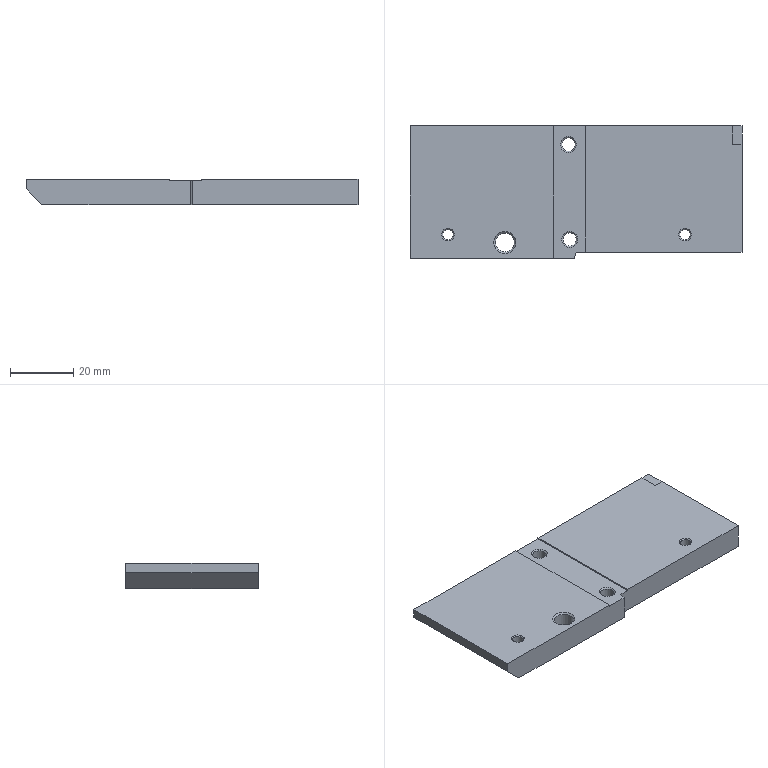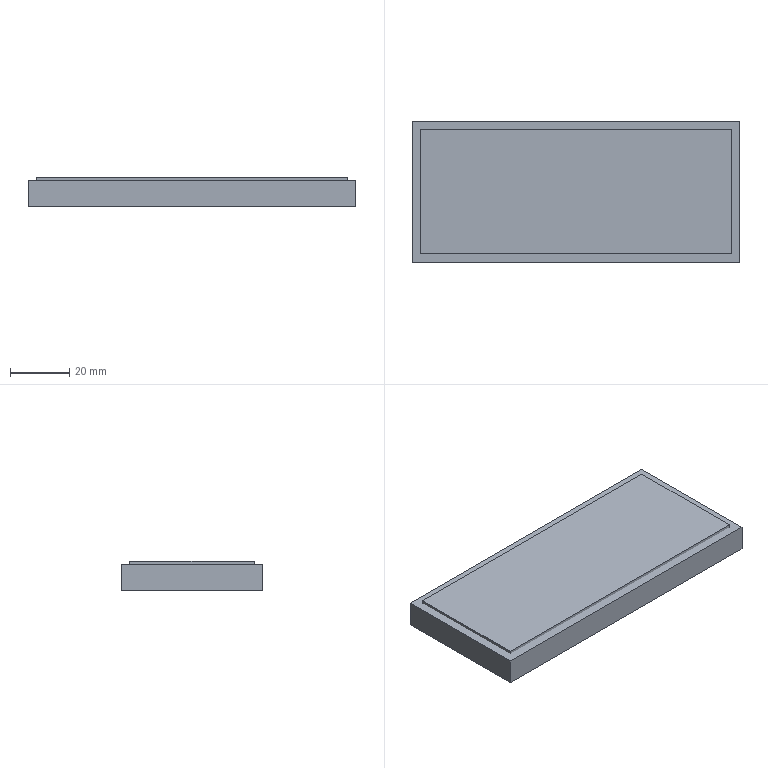CAM job | NX | 3+2 milling, drilling | part box 105 x 42 x 8 mm | stock box 111 x 48 x 10 mm
Tools:
number,name,description,diameter,corner_radius,flute_length,length,flutes
1,D50R0.8,Milling Tool-5 Parameters,50.0,0.8,50.0,75.0,2
2,ZXZ,Milling Tool-5 Parameters,6.0,0.0,50.0,75.0,2
13,3.3ZT,Drilling Tool,3.3,0.0,35.0,50.0,2
14,4.2ZT,Drilling Tool,4.2,0.0,35.0,50.0,2
16,6.0ZT,Drilling Tool,6.0,0.0,35.0,50.0,2
10,D10,Milling Tool-5 Parameters,10.0,0.0,50.0,75.0,2
4,D4,Milling Tool-5 Parameters,4.0,0.0,50.0,75.0,2
7,D6A45,Milling Tool-5 Parameters,6.0,0.0,3.0,3.0,2
6,D6,Milling Tool-5 Parameters,6.0,0.0,50.0,75.0,2
3,D2,Milling Tool-5 Parameters,2.0,0.0,50.0,75.0,2
5,D6R0.5,Milling Tool-5 Parameters,6.0,0.5,50.0,75.0,2
12,2.5ZT,Drilling Tool,2.5,0.0,35.0,50.0,2
Operations:
program,operation,operation_type,tool,method,geometry_group,spindle_rpm,surface_speed,feed_per_tooth,feed_cut,feed_plunge,cut_length_mm,path_length_mm,cut_time_min,machine_time_min
1磁台,FLOOR_WALL,VolumeBased25DMillingOperation,D50R0.8,METHOD,A,1200.0,188.0,0.4167,1000.0,100.0,173.0,227.0,0.173,0.1784
1磁台,DRILLING,Operation,ZXZ,METHOD,A,3000.0,56.0,0.0417,250.0,0.0,20.0,228.017,0.08,0.1008
1磁台,DRILLING_COPY,Operation,3.3ZT,METHOD,A,1929.0,20.0,0.0311,120.0,0.0,24.0,186.06,0.2,0.2162
1磁台,DRILLING_COPY_COPY,Operation,4.2ZT,METHOD,A,1929.0,20.0,0.0311,120.0,0.0,24.0,141.15,0.2,0.2117
1磁台,DRILLING_COPY_COPY_COPY,Operation,6.0ZT,METHOD,A,1929.0,20.0,0.0311,120.0,0.0,12.0,84.0,0.1,0.1072
1磁台,ZLEVEL_PROFILE,ZLevelMilling,D10,METHOD,A,3500.0,109.0,0.3143,2200.0,1000.0,13032.451,13097.451,5.942,5.948
1磁台,FLOOR_WALL_1_COPY,VolumeBased25DMillingOperation,D6,METHOD,A,4500.0,84.0,0.1611,1450.0,1000.0,206.171,269.74,0.1458,0.1521
1磁台,ZLEVEL_PROFILE_COPY,ZLevelMilling,D4,METHOD,A,4500.0,56.0,0.1667,1500.0,1000.0,456.934,813.067,0.3343,0.3699
1磁台,ZLEVEL_PROFILE_COPY_COPY_1,ZLevelMilling,D2,METHOD,A,5500.0,34.0,0.0909,1000.0,1000.0,594.675,1033.074,0.5947,0.6385
1磁台,ZLEVEL_PROFILE_COPY_COPY,ZLevelMilling,D4,METHOD,A,6500.0,81.0,0.0769,1000.0,1000.0,309.785,383.785,0.3098,0.3172
1磁台,ZLEVEL_PROFILE_COPY_COPY_COPY,ZLevelMilling,D6A45,METHOD,A,6500.0,81.0,0.0769,1000.0,1000.0,369.141,931.419,0.3691,0.4254
2虎钳,FLOOR_WALL_COPY,VolumeBased25DMillingOperation,D50R0.8,METHOD,B,1200.0,188.0,0.4167,1000.0,100.0,1002.0,2121.001,1.002,1.114
2虎钳,ZLEVEL_PROFILE_COPY_1,ZLevelMilling,D6R0.5,METHOD,B,6500.0,122.0,0.1692,2200.0,1000.0,3802.343,3864.914,1.73,1.736
2虎钳,ZLEVEL_PROFILE_COPY_COPY_COPY_COPY,ZLevelMilling,D6A45,METHOD,B,6500.0,81.0,0.0769,1000.0,1000.0,302.773,909.129,0.3028,0.3634
3,FLOOR_WALL_1_COPY_COPY,VolumeBased25DMillingOperation,D10,METHOD,C,4500.0,84.0,0.1611,1450.0,1000.0,678.909,1323.138,0.4898,0.5542
3,DRILLING_COPY_1,Operation,ZXZ,METHOD,C,3000.0,56.0,0.0417,250.0,0.0,20.0,252.893,0.08,0.1033
3,DRILLING_COPY_COPY_1,Operation,2.5ZT,METHOD,C,2000.0,15.0,0.03,120.0,0.0,63.004,276.82,0.525,0.5464
3,DRILLING_COPY_COPY_COPY_1,Operation,4.2ZT,METHOD,C,1929.0,20.0,0.0311,120.0,0.0,16.262,92.524,0.1355,0.1431
3,ZLEVEL_PROFILE_COPY_COPY_COPY_COPY_1,ZLevelMilling,D6A45,METHOD,C,6500.0,81.0,0.0769,1000.0,1000.0,270.263,793.68,0.2703,0.3226